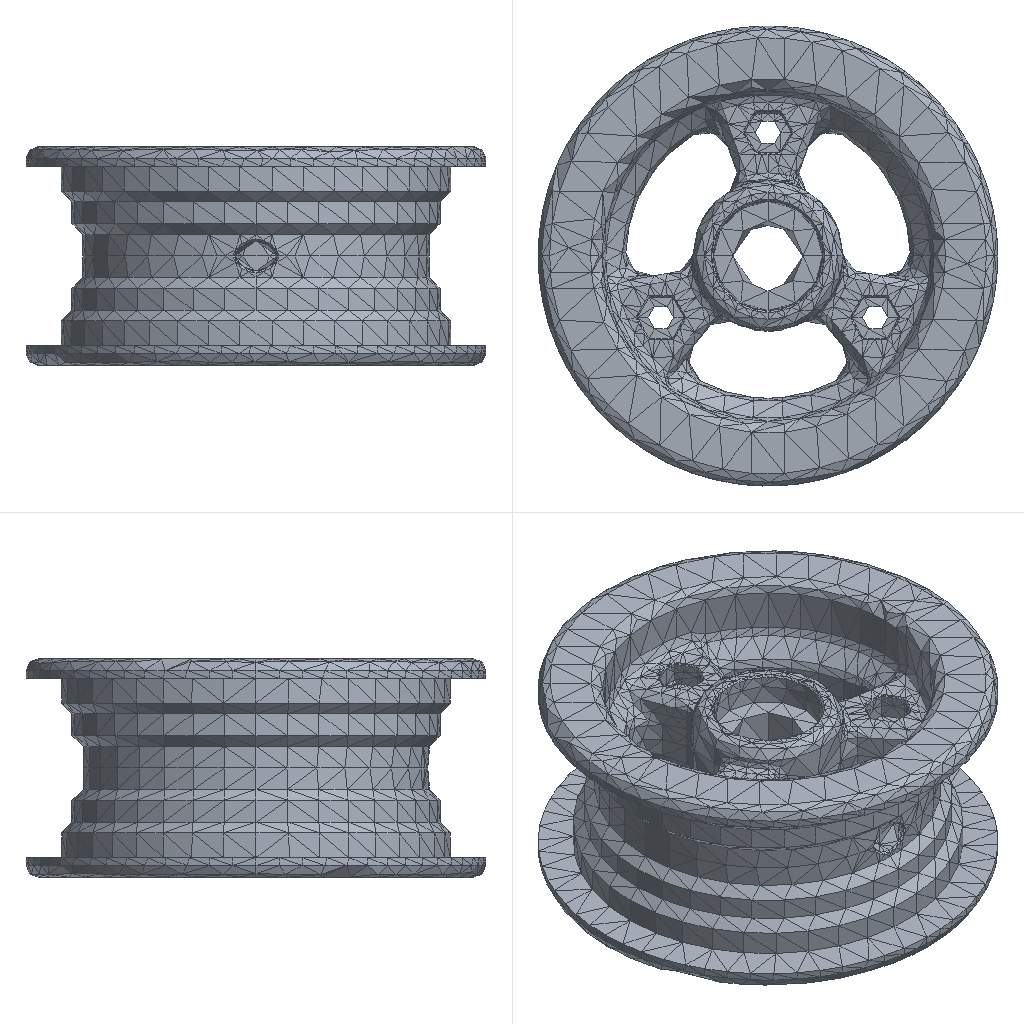Simulation study | ansys workbench
Ansys APDL input file, long lists of numbers shortened:
/batch
/config,noeldb,1     ! force off writing results to database
*get,_wallstrt,active,,time,wall
! ANSYS input file written by Workbench version 2022 R1
! File used for geometry attach:
/title,wbnew--____ (F5)
! ****** Begin Custom Load Command Snippet ******
/COM, ACT Extensions:
/COM,     LSDYNA, 2021.1
/COM,
! ****** End   Custom Load Command Snippet ******
*DIM,_wb_ProjectScratch_dir,string,248
_wb_ProjectScratch_dir(1) = ''
*DIM,_wb_SolverFiles_dir,string,248
_wb_SolverFiles_dir(1) = ''
*DIM,_wb_userfiles_dir,string,248
_wb_userfiles_dir(1) = ''
/com,--- Data in consistent NMM units. See Solving Units in the help system for more information.
/units,MPA
/nopr
/wb,file,start              !  signify a WB generated input file
/prep7
! Turn off shape checking because checks already performed inside WB mesher.
! See help system for more information.
SHPP,OFF,,NOWARN
/nolist
etcon,set             ! allow ANSYS to choose best KEYOP's for 180x elements, resets any applicable keyopt to MAPDL defaults
/com,*********** Nodes for the whole assembly ***********
nblock,3,,26501
(1i9,3e20.9e3)
        1    -5.769107078E+01    -3.299351067E+01     2.580641396E+01
! (24091 more lines like these left out)
-1
/com,*********** Nodes for all Remote Points ***********
nblock,3
(1i9,3e20.9e3)
    24093    -5.164832538E+01     2.922658694E+01     3.074033262E+01
-1
/wb,elem,start            !  set before creation of elements
/com,*********** Elements for Body 1 "Wheel Hub|NONE" ***********
et,1,187
eblock,19,solid,,6435
(19i9)
        1        1        1        1        0        0        0        0       10        0     6436    13672    13675    14007    13974    23210    23231    23216    23215
! (12869 more lines like these left out)
-1
/com,*********** Elements for Body 2 "Wheel Hub|NONE[2]" ***********
et,2,187
eblock,19,solid,,6435
(19i9)
        2        2        2        2        0        0        0        0       10        0        1     1626     1629     1961     1928    11164    11185    11170    11169
! (12869 more lines like these left out)
-1
/wb,elem,end               !  done creating elements
/com,*********** Send User Defined Coordinate System(s) ***********
csys,0
toffst,273.15,  ! Temperature offset from absolute zero
/com,*********** Set Reference Temperature ***********
tref,22.
/wb,mat,start              !  starting to send materials
/com,*********** Send Materials ***********
Temperature = 'TEMP' ! Temperature
MP,DENS,1,7.85e-09,	! tonne mm^-3
MP,ALPX,1,1.2e-05,	! C^-1
MP,C,1,434000000,	! mm^2 s^-2 C^-1
MP,KXX,1,60.5,	! tonne mm s^-3 C^-1
MP,RSVX,1,0.00017,	! ohm mm
MP,EX,1,200000,	! tonne s^-2 mm^-1
MP,NUXY,1,0.3,
MP,MURX,1,10000,
Temperature = 'TEMP' ! Temperature
MP,DENS,2,7.85e-09,	! tonne mm^-3
MP,ALPX,2,1.2e-05,	! C^-1
MP,C,2,434000000,	! mm^2 s^-2 C^-1
MP,KXX,2,60.5,	! tonne mm s^-3 C^-1
MP,RSVX,2,0.00017,	! ohm mm
MP,EX,2,200000,	! tonne s^-2 mm^-1
MP,NUXY,2,0.3,
MP,MURX,2,10000,
/wb,mat,end                !  done sending materials
!************************* Model Summary ********************
!Wheel Hub|NONE,	结构钢,	matid,	1
!Wheel Hub|NONE[2],	结构钢,	matid,	2
!************************* End Model Summary ********************
! get the diagonal of the bounding box. Needed later for other things
*get,_xmin,node,,mnloc,x
*get,_ymin,node,,mnloc,y
*get,_zmin,node,,mnloc,z
*get,_xmax,node,,mxloc,x
*get,_ymax,node,,mxloc,y
*get,_zmax,node,,mxloc,z
_ASMDIAG=(_xmax-_xmin)*(_xmax-_xmin)+(_ymax-_ymin)*(_ymax-_ymin)+(_zmax-_zmin)*(_zmax-_zmin)
_ASMDIAG=SQRT(_ASMDIAG)
/wb,contact,start          !  starting to send contact
/com,*********** Create Contact "接触区域" ***********
/com,            Real Constant Set For Above Contact Is 4 & 3
*set,tid,4
*set,cid,3
r,tid
r,cid
et,tid,170
et,cid,174
eblock,10,,,300
(15i9)
    19468        4        4        4        0    12085    12090    12091    12091    14250    14290    12091    14251
! (299 more lines like these left out)
-1
eblock,10,,,300
(15i9)
    19768        3        3        3        0    12085    12090    12091    12091    14250    14290    12091    14251
! (299 more lines like these left out)
-1
eblock,10,,,300
(15i9)
    20068        3        4        3        0       59      955     1125     1125     2337     8518     1125     2338
! (299 more lines like these left out)
-1
eblock,10,,,300
(15i9)
    20368        4        3        4        0       59      955     1125     1125     2337     8518     1125     2338
! (299 more lines like these left out)
-1
keyo,cid,8,2               ! auto create asymmetric contact (from Program Controlled setting)
keyo,cid,10,0              ! adjust contact stiffness each NR iteration (from Program Controlled setting)
keyo,cid,12,5              ! bonded always
keyo,cid,18,1              ! small sliding turned on by application
keyo,cid,2,0               ! augmented Lagrange (from Program Controlled setting)
keyo,cid,4,0               ! on Gauss point (from Program Controlled setting)
keyo,cid,9,1               ! ignore initial gaps/penetration
keyo,cid,7,0               ! No Prediction
rmod,tid,3,10.      ! FKN
rmod,tid,5,0.       ! ICONT
rmod,tid,6,0.       ! PINB
rmod,tid,10,0.      ! CNOF
rmod,tid,12,0.      ! FKT
rmod,tid,36,29      ! WB DSID
rmod,cid,3,10.      ! FKN
rmod,cid,5,0.       ! ICONT
rmod,cid,6,0.       ! PINB
rmod,cid,10,0.      ! CNOF
rmod,cid,12,0.      ! FKT
rmod,cid,36,29      ! WB DSID
nsel,all
esel,all
/wb,contact,end            !  done creating contacts
/golist
/wb,load,start             !  starting to send loads
/com,*********** Fixed Supports ***********
CMBLOCK,_FIXEDSU,NODE,      128
(8i10)
       823       824       825       826       827       828       829       830
! (15 more lines like these left out)
cmsel,s,_FIXEDSU
d,all,all
nsel,all
/com,*********** Create Remote Point "内部远程点" ***********
! -------- Remote Point Used by "力矩" --------
*set,tid,6
*set,cid,5
et,cid,174
et,tid,170
keyo,tid,2,1               ! Don't fix the pilot node
keyo,tid,4,111111
keyo,cid,12,5              ! Bonded Contact
keyo,cid,4,1               ! Deformable RBE3 style load
keyo,cid,2,2               ! MPC style contact
eblock,10,,,279
(15i9)
    20668        5        5        5        0    12306    13197    12192    12192    15842    14995    12192    14991
! (278 more lines like these left out)
-1
*set,_npilot,24093
_npilot40=_npilot
type,tid
mat ,cid
real,cid
tshape,pilo
en,20947,_npilot
tshape
/com,*********** Construct Moment Using Remote Attachment ***********
/gst,on,on
fini
*get,_numnode,node,0,count
*get,_numelem,elem,0,count
*get, _MAXELEMNUM, elem, 0, NUM, MAX
*get, _MAXNODENUM, node, 0, NUM, MAX
*get, _MAXELEMTYPE, etyp, 0, NUM, MAX
*get, _MAXREALCONST, real, 0, NUM, MAX
/go
/wb,load,end               !  done creating loads
/com,--- Number of total nodes = %_numnode%
/com,--- Number of contact elements = 1479
/com,--- Number of spring elements = 0
/com,--- Number of bearing elements = 0
/com,--- Number of solid elements = 12870
/com,--- Number of condensed parts = 0
/com,--- Number of total elements = %_numelem%
*get,_wallbsol,active,,time,wall
/com,****************************************************************************
/com,*************************    SOLUTION       ********************************
/com,****************************************************************************
/solu
antype,0                   ! static analysis
_thickRatio=  1     ! Ratio of thick parts in the model
eqsl,pcg,1e-8,,,,,,1
cntr,print,1               ! print out contact info and also make no initial contact an error
dmpoption,emat,no             ! Don't combine emat file for DANSYS
dmpoption,esav,no             ! Don't combine esav file for DANSYS
nldiag,cont,iter           ! print out contact info each equilibrium iteration
rescontrol,,none                 ! Do not keep any restart files
/com,****************************************************
/com,******************* SOLVE FOR LS 1 OF 1 ****************
nsel,s,node,,24093
f,all,mx,0.
f,all,my,0.
f,all,mz,5000.
nsel,all
/nopr
/gopr
nsub,1,1,1
time,1.
outres,erase
outres,all,none
outres,nsol,all,
outres,rsol,all
outres,eangl,all
outres,etmp,all
outres,veng,all
outres,strs,all,
outres,epel,all,
outres,eppl,all,
outres,cont,all,
! *********** WB SOLVE COMMAND ***********
! check interactive state
*get,ANSINTER_,active,,int
*if,ANSINTER_,ne,0,then
/eof
*endif
solve
/com *************** Write FE CONNECTORS *********
CEWRITE,file,ce,,INTE
/com,****************************************************
/com,*************** FINISHED SOLVE FOR LS 1 *************
*get,_wallasol,active,,time,wall
/nopr
*get,_numnode,node,0,count
*get,_numelem,elem,0,count
*get, _MAXELEMNUM, elem, 0, NUM, MAX
*get, _MAXNODENUM, node, 0, NUM, MAX,,,INTERNAL
*get, _MAXELEMTYPE, etyp, 0, NUM, MAX
*get, _MAXREALCONST, real, 0, NUM, MAX
/gopr
*get,_PCGITER,active,,solu,cgiter
/post1
xmlo,ENCODING,ISO-8859-1
xmlo,parm
/xml,parm,xml
fini
/gopr
*get,_walldone,active,,time,wall
_preptime=(_wallbsol-_wallstrt)*3600
_solvtime=(_wallasol-_wallbsol)*3600
_posttime=(_walldone-_wallasol)*3600
_totaltim=(_walldone-_wallstrt)*3600
*get,_dlbratio,active,0,solu,dlbr
*get,_combtime,active,0,solu,comb
*get,_ssmode,active,0,solu,ssmm
*get,_ndofs,active,0,solu,ndof
*get,_sol_end_time,active,0,set,time
*if,_sol_end_time,eq,1.,then
/fclean				!clean distributed files
*endif
/com,--- Total number of nodes = %_numnode%
/com,--- Total number of elements = %_numelem%
/com,--- Element load balance ratio = %_dlbratio%
/com,--- Time to combine distributed files = %_combtime%
/com,--- Sparse memory mode = %_ssmode%
/com,--- Number of DOF = %_ndofs%
/wb,file,end               ! done with WB generated input